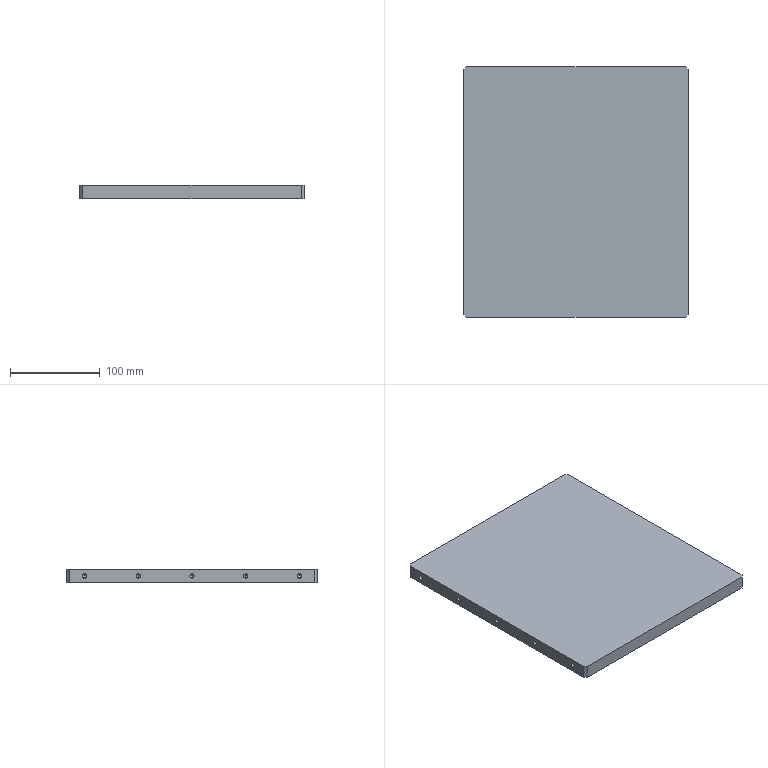Part | STEP file | 10-13 lift fixing plate B | 1 solid | 118 faces | box 250 x 280 x 15 mm | volume 1044782 mm3 | cylinder 56 | cone 48 | plane 14 | commonest cylinder face diameters 3.3 x20 5 x20 4 x8 4.2 x8